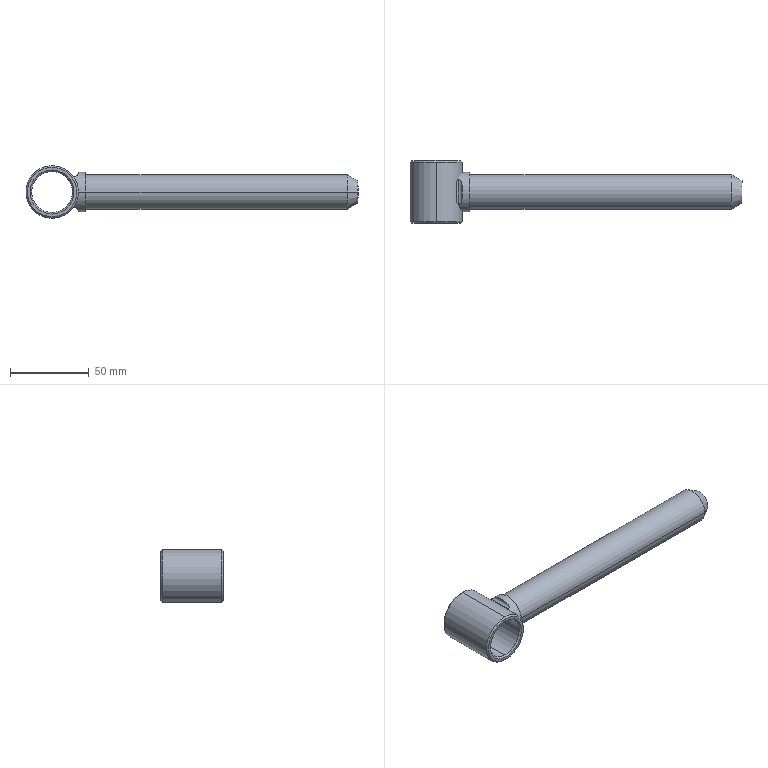Part | SolidWorks | features BaseBody 1 | 1 solid | 28 faces | box 211.2 x 40 x 33.4 mm | volume 81310 mm3 | cylinder 12 | cone 10 | plane 6 | commonest cylinder face diameters 4 x4 22 x2 25 x2 26.04 x2 33.4 x2
STEP:
#1=CARTESIAN_POINT('',(-54.286,20.854,0.));
#2=VERTEX_POINT('',#1);
#3=CARTESIAN_POINT('',(-54.286,-1.146,0.));
#4=VERTEX_POINT('',#3);
#5=CARTESIAN_POINT('',(-54.286,9.854,0.));
#6=DIRECTION('',(1.,0.,0.));
#7=DIRECTION('',(0.,1.,0.));
#8=AXIS2_PLACEMENT_3D('',#5,#6,#7);
#9=CIRCLE('',#8,11.);
#10=EDGE_CURVE('',#2,#4,#9,.T.);
#11=ORIENTED_EDGE('',*,*,#10,.T.);
#12=CARTESIAN_POINT('',(111.982,-1.146,0.));
#13=VERTEX_POINT('',#12);
#14=CARTESIAN_POINT('',(28.848,-1.146,0.));
#15=DIRECTION('',(1.,0.,0.));
#16=VECTOR('',#15,1000.);
#17=LINE('',#14,#16);
#18=EDGE_CURVE('',#4,#13,#17,.T.);
#19=ORIENTED_EDGE('',*,*,#18,.T.);
#20=CARTESIAN_POINT('',(111.982,20.854,0.));
#21=VERTEX_POINT('',#20);
#22=CARTESIAN_POINT('',(111.982,9.854,0.));
#23=DIRECTION('',(-1.,0.,0.));
#24=DIRECTION('',(0.,1.,0.));
#25=AXIS2_PLACEMENT_3D('',#22,#23,#24);
#26=CIRCLE('',#25,11.);
#27=EDGE_CURVE('',#13,#21,#26,.T.);
#28=ORIENTED_EDGE('',*,*,#27,.T.);
#29=CARTESIAN_POINT('',(28.848,20.854,0.));
#30=DIRECTION('',(1.,0.,0.));
#31=VECTOR('',#30,1000.);
#32=LINE('',#29,#31);
#33=EDGE_CURVE('',#2,#21,#32,.T.);
#34=ORIENTED_EDGE('',*,*,#33,.F.);
#35=EDGE_LOOP('',(#11,#19,#28,#34));
#36=FACE_OUTER_BOUND('',#35,.T.);
#37=CARTESIAN_POINT('',(28.848,9.854,0.));
#38=DIRECTION('',(1.,0.,0.));
#39=DIRECTION('',(0.,1.,0.));
#40=AXIS2_PLACEMENT_3D('',#37,#38,#39);
#41=CYLINDRICAL_SURFACE('',#40,11.);
#42=ADVANCED_FACE('',(#36),#41,.T.);
#43=CARTESIAN_POINT('',(118.714,2.741,0.));
#44=VERTEX_POINT('',#43);
#45=CARTESIAN_POINT('',(118.714,16.967,0.));
#46=VERTEX_POINT('',#45);
#47=CARTESIAN_POINT('',(118.714,9.854,0.));
#48=DIRECTION('',(-1.,0.,0.));
#49=DIRECTION('',(0.,-1.,0.));
#50=AXIS2_PLACEMENT_3D('',#47,#48,#49);
#51=CIRCLE('',#50,7.113);
#52=EDGE_CURVE('',#44,#46,#51,.T.);
#53=ORIENTED_EDGE('',*,*,#52,.T.);
#54=CARTESIAN_POINT('',(111.982,20.854,0.));
#55=DIRECTION('',(-0.866,0.5,0.));
#56=VECTOR('',#55,1000.);
#57=LINE('',#54,#56);
#58=EDGE_CURVE('',#46,#21,#57,.T.);
#59=ORIENTED_EDGE('',*,*,#58,.T.);
#60=ORIENTED_EDGE('',*,*,#27,.F.);
#61=CARTESIAN_POINT('',(111.982,-1.146,0.));
#62=DIRECTION('',(-0.866,-0.5,0.));
#63=VECTOR('',#62,1000.);
#64=LINE('',#61,#63);
#65=EDGE_CURVE('',#44,#13,#64,.T.);
#66=ORIENTED_EDGE('',*,*,#65,.F.);
#67=EDGE_LOOP('',(#53,#59,#60,#66));
#68=FACE_OUTER_BOUND('',#67,.T.);
#69=CARTESIAN_POINT('',(111.982,9.854,0.));
#70=DIRECTION('',(-1.,0.,0.));
#71=DIRECTION('',(0.,-1.,0.));
#72=AXIS2_PLACEMENT_3D('',#69,#70,#71);
#73=CONICAL_SURFACE('',#72,11.,0.5236);
#74=ADVANCED_FACE('',(#68),#73,.T.);
#75=CARTESIAN_POINT('',(-62.837,3.143,10.546));
#76=VERTEX_POINT('',#75);
#77=CARTESIAN_POINT('',(-59.086,-2.646,0.));
#78=VERTEX_POINT('',#77);
#79=CARTESIAN_POINT('',(-62.837,3.143,10.546));
#80=CARTESIAN_POINT('',(-62.392,2.286,10.));
#81=CARTESIAN_POINT('',(-61.935,1.517,9.368));
#82=CARTESIAN_POINT('',(-61.276,0.4757,8.279));
#83=CARTESIAN_POINT('',(-61.061,0.1469,7.892));
#84=CARTESIAN_POINT('',(-60.648,-0.4685,7.068));
#85=CARTESIAN_POINT('',(-60.454,-0.7505,6.638));
#86=CARTESIAN_POINT('',(-60.095,-1.263,5.738));
#87=CARTESIAN_POINT('',(-59.931,-1.494,5.269));
#88=CARTESIAN_POINT('',(-59.638,-1.9,4.288));
#89=CARTESIAN_POINT('',(-59.509,-2.075,3.774));
#90=CARTESIAN_POINT('',(-59.3,-2.358,2.722));
#91=CARTESIAN_POINT('',(-59.22,-2.466,2.181));
#92=CARTESIAN_POINT('',(-59.113,-2.61,1.096));
#93=CARTESIAN_POINT('',(-59.086,-2.646,0.5502));
#94=CARTESIAN_POINT('',(-59.086,-2.646,0.));
#95=B_SPLINE_CURVE_WITH_KNOTS('',3,(#79,#80,#81,#82,#83,#84,#85,#86,#87,#88,#89,#90,#91,#92,#93,#94),.UNSPECIFIED.,.F.,.F.,(4,2,2,2,2,2,2,4),(0.,0.003282,0.004923,0.006564,0.008205,0.009846,0.01149,0.01313),.UNSPECIFIED.);
#96=EDGE_CURVE('',#76,#78,#95,.T.);
#97=ORIENTED_EDGE('',*,*,#96,.T.);
#98=CARTESIAN_POINT('',(-54.286,-2.646,0.));
#99=VERTEX_POINT('',#98);
#100=CARTESIAN_POINT('',(-56.786,-2.646,0.));
#101=DIRECTION('',(1.,0.,0.));
#102=VECTOR('',#101,1000.);
#103=LINE('',#100,#102);
#104=EDGE_CURVE('',#78,#99,#103,.T.);
#105=ORIENTED_EDGE('',*,*,#104,.T.);
#106=CARTESIAN_POINT('',(-54.286,22.354,0.));
#107=VERTEX_POINT('',#106);
#108=CARTESIAN_POINT('',(-54.286,9.854,0.));
#109=DIRECTION('',(1.,0.,0.));
#110=DIRECTION('',(0.,1.,0.));
#111=AXIS2_PLACEMENT_3D('',#108,#109,#110);
#112=CIRCLE('',#111,12.5);
#113=EDGE_CURVE('',#107,#99,#112,.T.);
#114=ORIENTED_EDGE('',*,*,#113,.F.);
#115=CARTESIAN_POINT('',(-59.086,22.354,0.));
#116=VERTEX_POINT('',#115);
#117=CARTESIAN_POINT('',(-56.786,22.354,0.));
#118=DIRECTION('',(1.,0.,0.));
#119=VECTOR('',#118,1000.);
#120=LINE('',#117,#119);
#121=EDGE_CURVE('',#116,#107,#120,.T.);
#122=ORIENTED_EDGE('',*,*,#121,.F.);
#123=CARTESIAN_POINT('',(-62.837,16.565,10.546));
#124=VERTEX_POINT('',#123);
#125=CARTESIAN_POINT('',(-59.086,22.354,0.));
#126=CARTESIAN_POINT('',(-59.086,22.354,0.5493));
#127=CARTESIAN_POINT('',(-59.113,22.317,1.105));
#128=CARTESIAN_POINT('',(-59.222,22.172,2.197));
#129=CARTESIAN_POINT('',(-59.303,22.062,2.738));
#130=CARTESIAN_POINT('',(-59.614,21.64,4.301));
#131=CARTESIAN_POINT('',(-59.909,21.236,5.271));
#132=CARTESIAN_POINT('',(-60.452,20.461,6.634));
#133=CARTESIAN_POINT('',(-60.647,20.178,7.065));
#134=CARTESIAN_POINT('',(-61.055,19.57,7.881));
#135=CARTESIAN_POINT('',(-61.269,19.244,8.266));
#136=CARTESIAN_POINT('',(-61.709,18.549,8.995));
#137=CARTESIAN_POINT('',(-61.936,18.178,9.339));
#138=CARTESIAN_POINT('',(-62.389,17.4,9.978));
#139=CARTESIAN_POINT('',(-62.615,16.993,10.273));
#140=CARTESIAN_POINT('',(-62.837,16.565,10.546));
#141=B_SPLINE_CURVE_WITH_KNOTS('',3,(#125,#126,#127,#128,#129,#130,#131,#132,#133,#134,#135,#136,#137,#138,#139,#140),.UNSPECIFIED.,.F.,.F.,(4,2,2,2,2,2,2,4),(-0.00257,-0.0009334,0.0007035,0.003977,0.005614,0.007251,0.008888,0.01052),.UNSPECIFIED.);
#142=EDGE_CURVE('',#116,#124,#141,.T.);
#143=ORIENTED_EDGE('',*,*,#142,.T.);
#144=CARTESIAN_POINT('',(-61.286,17.603,9.808));
#145=VERTEX_POINT('',#144);
#146=CARTESIAN_POINT('',(-62.837,16.565,10.546));
#147=CARTESIAN_POINT('',(-62.765,16.703,10.458));
#148=CARTESIAN_POINT('',(-62.683,16.832,10.372));
#149=CARTESIAN_POINT('',(-62.49,17.072,10.206));
#150=CARTESIAN_POINT('',(-62.378,17.184,10.126));
#151=CARTESIAN_POINT('',(-62.115,17.379,9.982));
#152=CARTESIAN_POINT('',(-61.967,17.459,9.92));
#153=CARTESIAN_POINT('',(-61.722,17.544,9.855));
#154=CARTESIAN_POINT('',(-61.638,17.566,9.838));
#155=CARTESIAN_POINT('',(-61.465,17.595,9.815));
#156=CARTESIAN_POINT('',(-61.375,17.603,9.808));
#157=CARTESIAN_POINT('',(-61.286,17.603,9.808));
#158=B_SPLINE_CURVE_WITH_KNOTS('',3,(#146,#147,#148,#149,#150,#151,#152,#153,#154,#155,#156,#157),.UNSPECIFIED.,.F.,.F.,(4,2,2,2,2,4),(0.,0.0005249,0.00105,0.001575,0.001837,0.0021),.UNSPECIFIED.);
#159=EDGE_CURVE('',#124,#145,#158,.T.);
#160=ORIENTED_EDGE('',*,*,#159,.T.);
#161=CARTESIAN_POINT('',(-59.286,13.954,11.808));
#162=VERTEX_POINT('',#161);
#163=CARTESIAN_POINT('',(-61.286,17.603,9.808));
#164=CARTESIAN_POINT('',(-61.073,17.603,9.808));
#165=CARTESIAN_POINT('',(-60.861,17.558,9.844));
#166=CARTESIAN_POINT('',(-60.579,17.44,9.935));
#167=CARTESIAN_POINT('',(-60.489,17.392,9.972));
#168=CARTESIAN_POINT('',(-60.325,17.284,10.052));
#169=CARTESIAN_POINT('',(-60.249,17.225,10.096));
#170=CARTESIAN_POINT('',(-60.038,17.03,10.236));
#171=CARTESIAN_POINT('',(-59.922,16.882,10.339));
#172=CARTESIAN_POINT('',(-59.729,16.568,10.545));
#173=CARTESIAN_POINT('',(-59.65,16.399,10.651));
#174=CARTESIAN_POINT('',(-59.459,15.878,10.96));
#175=CARTESIAN_POINT('',(-59.387,15.512,11.154));
#176=CARTESIAN_POINT('',(-59.3,14.748,11.51));
#177=CARTESIAN_POINT('',(-59.286,14.355,11.669));
#178=CARTESIAN_POINT('',(-59.286,13.954,11.808));
#179=B_SPLINE_CURVE_WITH_KNOTS('',3,(#163,#164,#165,#166,#167,#168,#169,#170,#171,#172,#173,#174,#175,#176,#177,#178),.UNSPECIFIED.,.F.,.F.,(4,2,2,2,2,2,2,4),(0.0021,0.002728,0.003041,0.003355,0.003983,0.004611,0.005867,0.007122),.UNSPECIFIED.);
#180=EDGE_CURVE('',#145,#162,#179,.T.);
#181=ORIENTED_EDGE('',*,*,#180,.T.);
#182=CARTESIAN_POINT('',(-59.286,5.754,11.808));
#183=VERTEX_POINT('',#182);
#184=CARTESIAN_POINT('',(-59.286,9.854,0.));
#185=DIRECTION('',(1.,0.,0.));
#186=DIRECTION('',(0.,1.,0.));
#187=AXIS2_PLACEMENT_3D('',#184,#185,#186);
#188=CIRCLE('',#187,12.5);
#189=EDGE_CURVE('',#162,#183,#188,.T.);
#190=ORIENTED_EDGE('',*,*,#189,.T.);
#191=CARTESIAN_POINT('',(-61.286,2.105,9.808));
#192=VERTEX_POINT('',#191);
#193=CARTESIAN_POINT('',(-59.286,5.754,11.808));
#194=CARTESIAN_POINT('',(-59.286,5.354,11.669));
#195=CARTESIAN_POINT('',(-59.3,4.964,11.511));
#196=CARTESIAN_POINT('',(-59.385,4.209,11.161));
#197=CARTESIAN_POINT('',(-59.455,3.844,10.968));
#198=CARTESIAN_POINT('',(-59.646,3.317,10.657));
#199=CARTESIAN_POINT('',(-59.724,3.148,10.551));
#200=CARTESIAN_POINT('',(-59.916,2.834,10.344));
#201=CARTESIAN_POINT('',(-60.031,2.686,10.242));
#202=CARTESIAN_POINT('',(-60.243,2.488,10.1));
#203=CARTESIAN_POINT('',(-60.32,2.428,10.055));
#204=CARTESIAN_POINT('',(-60.485,2.318,9.973));
#205=CARTESIAN_POINT('',(-60.575,2.27,9.936));
#206=CARTESIAN_POINT('',(-60.764,2.19,9.875));
#207=CARTESIAN_POINT('',(-60.863,2.159,9.851));
#208=CARTESIAN_POINT('',(-61.072,2.116,9.817));
#209=CARTESIAN_POINT('',(-61.179,2.105,9.808));
#210=CARTESIAN_POINT('',(-61.286,2.105,9.808));
#211=B_SPLINE_CURVE_WITH_KNOTS('',3,(#193,#194,#195,#196,#197,#198,#199,#200,#201,#202,#203,#204,#205,#206,#207,#208,#209,#210),.UNSPECIFIED.,.F.,.F.,(4,2,2,2,2,2,2,2,4),(0.,0.001255,0.00251,0.003137,0.003765,0.004079,0.004392,0.004706,0.00502),.UNSPECIFIED.);
#212=EDGE_CURVE('',#183,#192,#211,.T.);
#213=ORIENTED_EDGE('',*,*,#212,.T.);
#214=CARTESIAN_POINT('',(-61.286,2.105,9.808));
#215=CARTESIAN_POINT('',(-61.462,2.105,9.808));
#216=CARTESIAN_POINT('',(-61.64,2.136,9.833));
#217=CARTESIAN_POINT('',(-61.965,2.248,9.92));
#218=CARTESIAN_POINT('',(-62.113,2.329,9.982));
#219=CARTESIAN_POINT('',(-62.374,2.521,10.124));
#220=CARTESIAN_POINT('',(-62.488,2.633,10.205));
#221=CARTESIAN_POINT('',(-62.682,2.875,10.371));
#222=CARTESIAN_POINT('',(-62.765,3.005,10.458));
#223=CARTESIAN_POINT('',(-62.837,3.143,10.546));
#224=B_SPLINE_CURVE_WITH_KNOTS('',3,(#214,#215,#216,#217,#218,#219,#220,#221,#222,#223),.UNSPECIFIED.,.F.,.F.,(4,2,2,2,4),(0.00502,0.005538,0.006055,0.006573,0.007091),.UNSPECIFIED.);
#225=EDGE_CURVE('',#192,#76,#224,.T.);
#226=ORIENTED_EDGE('',*,*,#225,.T.);
#227=EDGE_LOOP('',(#97,#105,#114,#122,#143,#160,#181,#190,#213,#226));
#228=FACE_OUTER_BOUND('',#227,.T.);
#229=CARTESIAN_POINT('',(-56.786,9.854,0.));
#230=DIRECTION('',(1.,0.,0.));
#231=DIRECTION('',(0.,1.,0.));
#232=AXIS2_PLACEMENT_3D('',#229,#230,#231);
#233=CYLINDRICAL_SURFACE('',#232,12.5);
#234=ADVANCED_FACE('',(#228),#233,.T.);
#235=CARTESIAN_POINT('',(-62.837,16.565,-10.546));
#236=VERTEX_POINT('',#235);
#237=CARTESIAN_POINT('',(-62.837,3.143,-10.546));
#238=VERTEX_POINT('',#237);
#239=CARTESIAN_POINT('',(-62.837,9.854,-10.546));
#240=DIRECTION('',(0.,-1.,0.));
#241=VECTOR('',#240,1000.);
#242=LINE('',#239,#241);
#243=EDGE_CURVE('',#236,#238,#242,.T.);
#244=ORIENTED_EDGE('',*,*,#243,.T.);
#245=CARTESIAN_POINT('',(-59.086,-2.646,0.));
#246=CARTESIAN_POINT('',(-59.086,-2.646,-0.5493));
#247=CARTESIAN_POINT('',(-59.113,-2.609,-1.105));
#248=CARTESIAN_POINT('',(-59.222,-2.464,-2.197));
#249=CARTESIAN_POINT('',(-59.303,-2.354,-2.738));
#250=CARTESIAN_POINT('',(-59.614,-1.932,-4.301));
#251=CARTESIAN_POINT('',(-59.909,-1.528,-5.271));
#252=CARTESIAN_POINT('',(-60.452,-0.753,-6.634));
#253=CARTESIAN_POINT('',(-60.647,-0.4702,-7.065));
#254=CARTESIAN_POINT('',(-61.055,0.138,-7.881));
#255=CARTESIAN_POINT('',(-61.269,0.4638,-8.266));
#256=CARTESIAN_POINT('',(-61.709,1.159,-8.995));
#257=CARTESIAN_POINT('',(-61.936,1.53,-9.339));
#258=CARTESIAN_POINT('',(-62.389,2.308,-9.978));
#259=CARTESIAN_POINT('',(-62.615,2.715,-10.273));
#260=CARTESIAN_POINT('',(-62.837,3.143,-10.546));
#261=B_SPLINE_CURVE_WITH_KNOTS('',3,(#245,#246,#247,#248,#249,#250,#251,#252,#253,#254,#255,#256,#257,#258,#259,#260),.UNSPECIFIED.,.F.,.F.,(4,2,2,2,2,2,2,4),(0.01313,0.01477,0.01641,0.01968,0.02132,0.02296,0.0246,0.02624),.UNSPECIFIED.);
#262=EDGE_CURVE('',#78,#238,#261,.T.);
#263=ORIENTED_EDGE('',*,*,#262,.F.);
#264=ORIENTED_EDGE('',*,*,#96,.F.);
#265=CARTESIAN_POINT('',(-62.837,9.854,10.546));
#266=DIRECTION('',(0.,1.,0.));
#267=VECTOR('',#266,1000.);
#268=LINE('',#265,#267);
#269=EDGE_CURVE('',#76,#124,#268,.T.);
#270=ORIENTED_EDGE('',*,*,#269,.T.);
#271=ORIENTED_EDGE('',*,*,#142,.F.);
#272=CARTESIAN_POINT('',(-62.837,16.565,-10.546));
#273=CARTESIAN_POINT('',(-62.392,17.422,-10.));
#274=CARTESIAN_POINT('',(-61.935,18.191,-9.368));
#275=CARTESIAN_POINT('',(-61.276,19.232,-8.279));
#276=CARTESIAN_POINT('',(-61.061,19.561,-7.892));
#277=CARTESIAN_POINT('',(-60.648,20.177,-7.068));
#278=CARTESIAN_POINT('',(-60.454,20.459,-6.638));
#279=CARTESIAN_POINT('',(-60.095,20.971,-5.738));
#280=CARTESIAN_POINT('',(-59.931,21.202,-5.269));
#281=CARTESIAN_POINT('',(-59.638,21.608,-4.288));
#282=CARTESIAN_POINT('',(-59.509,21.783,-3.774));
#283=CARTESIAN_POINT('',(-59.3,22.066,-2.722));
#284=CARTESIAN_POINT('',(-59.22,22.174,-2.181));
#285=CARTESIAN_POINT('',(-59.113,22.318,-1.096));
#286=CARTESIAN_POINT('',(-59.086,22.354,-0.5502));
#287=CARTESIAN_POINT('',(-59.086,22.354,0.));
#288=B_SPLINE_CURVE_WITH_KNOTS('',3,(#272,#273,#274,#275,#276,#277,#278,#279,#280,#281,#282,#283,#284,#285,#286,#287),.UNSPECIFIED.,.F.,.F.,(4,2,2,2,2,2,2,4),(-0.01569,-0.01241,-0.01077,-0.009129,-0.007489,-0.005849,-0.00421,-0.00257),.UNSPECIFIED.);
#289=EDGE_CURVE('',#236,#116,#288,.T.);
#290=ORIENTED_EDGE('',*,*,#289,.F.);
#291=EDGE_LOOP('',(#244,#263,#264,#270,#271,#290));
#292=FACE_BOUND('',#291,.T.);
#293=CARTESIAN_POINT('',(-75.786,-9.146,16.7));
#294=VERTEX_POINT('',#293);
#295=CARTESIAN_POINT('',(-75.786,-9.146,-16.7));
#296=VERTEX_POINT('',#295);
#297=CARTESIAN_POINT('',(-75.786,-9.146,0.));
#298=DIRECTION('',(0.,1.,0.));
#299=DIRECTION('',(0.,0.,1.));
#300=AXIS2_PLACEMENT_3D('',#297,#298,#299);
#301=CIRCLE('',#300,16.7);
#302=EDGE_CURVE('',#294,#296,#301,.T.);
#303=ORIENTED_EDGE('',*,*,#302,.T.);
#304=CARTESIAN_POINT('',(-75.786,28.854,-16.7));
#305=VERTEX_POINT('',#304);
#306=CARTESIAN_POINT('',(-75.786,9.854,-16.7));
#307=DIRECTION('',(0.,1.,0.));
#308=VECTOR('',#307,1000.);
#309=LINE('',#306,#308);
#310=EDGE_CURVE('',#296,#305,#309,.T.);
#311=ORIENTED_EDGE('',*,*,#310,.T.);
#312=CARTESIAN_POINT('',(-75.786,28.854,16.7));
#313=VERTEX_POINT('',#312);
#314=CARTESIAN_POINT('',(-75.786,28.854,0.));
#315=DIRECTION('',(0.,-1.,0.));
#316=DIRECTION('',(0.,0.,1.));
#317=AXIS2_PLACEMENT_3D('',#314,#315,#316);
#318=CIRCLE('',#317,16.7);
#319=EDGE_CURVE('',#305,#313,#318,.T.);
#320=ORIENTED_EDGE('',*,*,#319,.T.);
#321=CARTESIAN_POINT('',(-75.786,9.854,16.7));
#322=DIRECTION('',(0.,1.,0.));
#323=VECTOR('',#322,1000.);
#324=LINE('',#321,#323);
#325=EDGE_CURVE('',#294,#313,#324,.T.);
#326=ORIENTED_EDGE('',*,*,#325,.F.);
#327=EDGE_LOOP('',(#303,#311,#320,#326));
#328=FACE_OUTER_BOUND('',#327,.T.);
#329=CARTESIAN_POINT('',(-75.786,9.854,0.));
#330=DIRECTION('',(0.,1.,0.));
#331=DIRECTION('',(0.,0.,1.));
#332=AXIS2_PLACEMENT_3D('',#329,#330,#331);
#333=CYLINDRICAL_SURFACE('',#332,16.7);
#334=ADVANCED_FACE('',(#292,#328),#333,.T.);
#335=ORIENTED_EDGE('',*,*,#180,.F.);
#336=CARTESIAN_POINT('',(-61.286,9.854,9.808));
#337=DIRECTION('',(0.,-1.,0.));
#338=VECTOR('',#337,1000.);
#339=LINE('',#336,#338);
#340=EDGE_CURVE('',#145,#192,#339,.T.);
#341=ORIENTED_EDGE('',*,*,#340,.T.);
#342=ORIENTED_EDGE('',*,*,#212,.F.);
#343=CARTESIAN_POINT('',(-59.286,9.854,11.808));
#344=DIRECTION('',(0.,-1.,0.));
#345=VECTOR('',#344,1000.);
#346=LINE('',#343,#345);
#347=EDGE_CURVE('',#162,#183,#346,.T.);
#348=ORIENTED_EDGE('',*,*,#347,.F.);
#349=EDGE_LOOP('',(#335,#341,#342,#348));
#350=FACE_OUTER_BOUND('',#349,.T.);
#351=CARTESIAN_POINT('',(-61.286,9.854,11.808));
#352=DIRECTION('',(0.,-1.,0.));
#353=DIRECTION('',(0.,0.,-1.));
#354=AXIS2_PLACEMENT_3D('',#351,#352,#353);
#355=CYLINDRICAL_SURFACE('',#354,2.);
#356=ADVANCED_FACE('',(#350),#355,.F.);
#357=CARTESIAN_POINT('',(-61.286,2.105,-9.808));
#358=VERTEX_POINT('',#357);
#359=CARTESIAN_POINT('',(-59.286,5.754,-11.808));
#360=VERTEX_POINT('',#359);
#361=CARTESIAN_POINT('',(-61.286,2.105,-9.808));
#362=CARTESIAN_POINT('',(-61.073,2.105,-9.808));
#363=CARTESIAN_POINT('',(-60.861,2.15,-9.844));
#364=CARTESIAN_POINT('',(-60.579,2.268,-9.935));
#365=CARTESIAN_POINT('',(-60.489,2.316,-9.972));
#366=CARTESIAN_POINT('',(-60.325,2.424,-10.052));
#367=CARTESIAN_POINT('',(-60.249,2.483,-10.096));
#368=CARTESIAN_POINT('',(-60.038,2.678,-10.236));
#369=CARTESIAN_POINT('',(-59.922,2.826,-10.339));
#370=CARTESIAN_POINT('',(-59.729,3.14,-10.545));
#371=CARTESIAN_POINT('',(-59.65,3.309,-10.651));
#372=CARTESIAN_POINT('',(-59.459,3.83,-10.96));
#373=CARTESIAN_POINT('',(-59.387,4.196,-11.154));
#374=CARTESIAN_POINT('',(-59.3,4.96,-11.51));
#375=CARTESIAN_POINT('',(-59.286,5.353,-11.669));
#376=CARTESIAN_POINT('',(-59.286,5.754,-11.808));
#377=B_SPLINE_CURVE_WITH_KNOTS('',3,(#361,#362,#363,#364,#365,#366,#367,#368,#369,#370,#371,#372,#373,#374,#375,#376),.UNSPECIFIED.,.F.,.F.,(4,2,2,2,2,2,2,4),(0.0021,0.002728,0.003041,0.003355,0.003983,0.004611,0.005867,0.007122),.UNSPECIFIED.);
#378=EDGE_CURVE('',#358,#360,#377,.T.);
#379=ORIENTED_EDGE('',*,*,#378,.F.);
#380=CARTESIAN_POINT('',(-61.286,17.603,-9.808));
#381=VERTEX_POINT('',#380);
#382=CARTESIAN_POINT('',(-61.286,9.854,-9.808));
#383=DIRECTION('',(0.,1.,0.));
#384=VECTOR('',#383,1000.);
#385=LINE('',#382,#384);
#386=EDGE_CURVE('',#358,#381,#385,.T.);
#387=ORIENTED_EDGE('',*,*,#386,.T.);
#388=CARTESIAN_POINT('',(-59.286,13.954,-11.808));
#389=VERTEX_POINT('',#388);
#390=CARTESIAN_POINT('',(-59.286,13.954,-11.808));
#391=CARTESIAN_POINT('',(-59.286,14.354,-11.669));
#392=CARTESIAN_POINT('',(-59.3,14.744,-11.511));
#393=CARTESIAN_POINT('',(-59.385,15.499,-11.161));
#394=CARTESIAN_POINT('',(-59.455,15.864,-10.968));
#395=CARTESIAN_POINT('',(-59.646,16.391,-10.657));
#396=CARTESIAN_POINT('',(-59.724,16.56,-10.551));
#397=CARTESIAN_POINT('',(-59.916,16.874,-10.344));
#398=CARTESIAN_POINT('',(-60.031,17.022,-10.242));
#399=CARTESIAN_POINT('',(-60.243,17.22,-10.1));
#400=CARTESIAN_POINT('',(-60.32,17.28,-10.055));
#401=CARTESIAN_POINT('',(-60.485,17.39,-9.973));
#402=CARTESIAN_POINT('',(-60.575,17.438,-9.936));
#403=CARTESIAN_POINT('',(-60.764,17.518,-9.875));
#404=CARTESIAN_POINT('',(-60.863,17.549,-9.851));
#405=CARTESIAN_POINT('',(-61.072,17.592,-9.817));
#406=CARTESIAN_POINT('',(-61.179,17.603,-9.808));
#407=CARTESIAN_POINT('',(-61.286,17.603,-9.808));
#408=B_SPLINE_CURVE_WITH_KNOTS('',3,(#390,#391,#392,#393,#394,#395,#396,#397,#398,#399,#400,#401,#402,#403,#404,#405,#406,#407),.UNSPECIFIED.,.F.,.F.,(4,2,2,2,2,2,2,2,4),(0.,0.001255,0.00251,0.003137,0.003765,0.004079,0.004392,0.004706,0.00502),.UNSPECIFIED.);
#409=EDGE_CURVE('',#389,#381,#408,.T.);
#410=ORIENTED_EDGE('',*,*,#409,.F.);
#411=CARTESIAN_POINT('',(-59.286,9.854,-11.808));
#412=DIRECTION('',(0.,1.,0.));
#413=VECTOR('',#412,1000.);
#414=LINE('',#411,#413);
#415=EDGE_CURVE('',#360,#389,#414,.T.);
#416=ORIENTED_EDGE('',*,*,#415,.F.);
#417=EDGE_LOOP('',(#379,#387,#410,#416));
#418=FACE_OUTER_BOUND('',#417,.T.);
#419=CARTESIAN_POINT('',(-61.286,9.854,-11.808));
#420=DIRECTION('',(0.,1.,0.));
#421=DIRECTION('',(0.,0.,1.));
#422=AXIS2_PLACEMENT_3D('',#419,#420,#421);
#423=CYLINDRICAL_SURFACE('',#422,2.);
#424=ADVANCED_FACE('',(#418),#423,.F.);
#425=CARTESIAN_POINT('',(-75.786,-10.146,15.7));
#426=VERTEX_POINT('',#425);
#427=CARTESIAN_POINT('',(-75.786,-10.146,-15.7));
#428=VERTEX_POINT('',#427);
#429=CARTESIAN_POINT('',(-75.786,-10.146,0.));
#430=DIRECTION('',(0.,1.,0.));
#431=DIRECTION('',(0.,0.,1.));
#432=AXIS2_PLACEMENT_3D('',#429,#430,#431);
#433=CIRCLE('',#432,15.7);
#434=EDGE_CURVE('',#426,#428,#433,.T.);
#435=ORIENTED_EDGE('',*,*,#434,.T.);
#436=CARTESIAN_POINT('',(-75.786,-9.146,-16.7));
#437=DIRECTION('',(0.,0.7071,-0.7071));
#438=VECTOR('',#437,1000.);
#439=LINE('',#436,#438);
#440=EDGE_CURVE('',#428,#296,#439,.T.);
#441=ORIENTED_EDGE('',*,*,#440,.T.);
#442=ORIENTED_EDGE('',*,*,#302,.F.);
#443=CARTESIAN_POINT('',(-75.786,-9.146,16.7));
#444=DIRECTION('',(0.,0.7071,0.7071));
#445=VECTOR('',#444,1000.);
#446=LINE('',#443,#445);
#447=EDGE_CURVE('',#426,#294,#446,.T.);
#448=ORIENTED_EDGE('',*,*,#447,.F.);
#449=EDGE_LOOP('',(#435,#441,#442,#448));
#450=FACE_OUTER_BOUND('',#449,.T.);
#451=CARTESIAN_POINT('',(-75.786,-9.146,0.));
#452=DIRECTION('',(0.,1.,0.));
#453=DIRECTION('',(0.,0.,1.));
#454=AXIS2_PLACEMENT_3D('',#451,#452,#453);
#455=CONICAL_SURFACE('',#454,16.7,0.7854);
#456=ADVANCED_FACE('',(#450),#455,.T.);
#457=CARTESIAN_POINT('',(-75.786,29.854,-15.7));
#458=VERTEX_POINT('',#457);
#459=CARTESIAN_POINT('',(-75.786,29.854,15.7));
#460=VERTEX_POINT('',#459);
#461=CARTESIAN_POINT('',(-75.786,29.854,0.));
#462=DIRECTION('',(0.,-1.,0.));
#463=DIRECTION('',(0.,0.,-1.));
#464=AXIS2_PLACEMENT_3D('',#461,#462,#463);
#465=CIRCLE('',#464,15.7);
#466=EDGE_CURVE('',#458,#460,#465,.T.);
#467=ORIENTED_EDGE('',*,*,#466,.T.);
#468=CARTESIAN_POINT('',(-75.786,28.854,16.7));
#469=DIRECTION('',(0.,-0.7071,0.7071));
#470=VECTOR('',#469,1000.);
#471=LINE('',#468,#470);
#472=EDGE_CURVE('',#460,#313,#471,.T.);
#473=ORIENTED_EDGE('',*,*,#472,.T.);
#474=ORIENTED_EDGE('',*,*,#319,.F.);
#475=CARTESIAN_POINT('',(-75.786,28.854,-16.7));
#476=DIRECTION('',(0.,-0.7071,-0.7071));
#477=VECTOR('',#476,1000.);
#478=LINE('',#475,#477);
#479=EDGE_CURVE('',#458,#305,#478,.T.);
#480=ORIENTED_EDGE('',*,*,#479,.F.);
#481=EDGE_LOOP('',(#467,#473,#474,#480));
#482=FACE_OUTER_BOUND('',#481,.T.);
#483=CARTESIAN_POINT('',(-75.786,28.854,0.));
#484=DIRECTION('',(0.,-1.,0.));
#485=DIRECTION('',(0.,0.,-1.));
#486=AXIS2_PLACEMENT_3D('',#483,#484,#485);
#487=CONICAL_SURFACE('',#486,16.7,0.7854);
#488=ADVANCED_FACE('',(#482),#487,.T.);
#489=CARTESIAN_POINT('',(-75.786,-9.146,13.02));
#490=VERTEX_POINT('',#489);
#491=CARTESIAN_POINT('',(-75.786,-9.146,-13.02));
#492=VERTEX_POINT('',#491);
#493=CARTESIAN_POINT('',(-75.786,-9.146,0.));
#494=DIRECTION('',(0.,-1.,0.));
#495=DIRECTION('',(1.,0.,0.));
#496=AXIS2_PLACEMENT_3D('',#493,#494,#495);
#497=CIRCLE('',#496,13.02);
#498=EDGE_CURVE('',#490,#492,#497,.T.);
#499=ORIENTED_EDGE('',*,*,#498,.F.);
#500=CARTESIAN_POINT('',(-75.786,-10.146,14.02));
#501=VERTEX_POINT('',#500);
#502=CARTESIAN_POINT('',(-75.786,-10.146,14.02));
#503=DIRECTION('',(0.,-0.7071,0.7071));
#504=VECTOR('',#503,1000.);
#505=LINE('',#502,#504);
#506=EDGE_CURVE('',#490,#501,#505,.T.);
#507=ORIENTED_EDGE('',*,*,#506,.T.);
#508=CARTESIAN_POINT('',(-75.786,-10.146,-14.02));
#509=VERTEX_POINT('',#508);
#510=CARTESIAN_POINT('',(-75.786,-10.146,0.));
#511=DIRECTION('',(0.,1.,0.));
#512=DIRECTION('',(0.,0.,-1.));
#513=AXIS2_PLACEMENT_3D('',#510,#511,#512);
#514=CIRCLE('',#513,14.02);
#515=EDGE_CURVE('',#509,#501,#514,.T.);
#516=ORIENTED_EDGE('',*,*,#515,.F.);
#517=CARTESIAN_POINT('',(-75.786,-10.146,-14.02));
#518=DIRECTION('',(0.,-0.7071,-0.7071));
#519=VECTOR('',#518,1000.);
#520=LINE('',#517,#519);
#521=EDGE_CURVE('',#492,#509,#520,.T.);
#522=ORIENTED_EDGE('',*,*,#521,.F.);
#523=EDGE_LOOP('',(#499,#507,#516,#522));
#524=FACE_OUTER_BOUND('',#523,.T.);
#525=CARTESIAN_POINT('',(-75.786,-10.146,0.));
#526=DIRECTION('',(0.,-1.,0.));
#527=DIRECTION('',(0.,0.,-1.));
#528=AXIS2_PLACEMENT_3D('',#525,#526,#527);
#529=CONICAL_SURFACE('',#528,14.02,0.7854);
#530=ADVANCED_FACE('',(#524),#529,.F.);
#531=CARTESIAN_POINT('',(-75.786,28.854,-13.02));
#532=VERTEX_POINT('',#531);
#533=CARTESIAN_POINT('',(-75.786,28.854,13.02));
#534=VERTEX_POINT('',#533);
#535=CARTESIAN_POINT('',(-75.786,28.854,0.));
#536=DIRECTION('',(0.,1.,0.));
#537=DIRECTION('',(1.,0.,0.));
#538=AXIS2_PLACEMENT_3D('',#535,#536,#537);
#539=CIRCLE('',#538,13.02);
#540=EDGE_CURVE('',#532,#534,#539,.T.);
#541=ORIENTED_EDGE('',*,*,#540,.F.);
#542=CARTESIAN_POINT('',(-75.786,29.854,-14.02));
#543=VERTEX_POINT('',#542);
#544=CARTESIAN_POINT('',(-75.786,29.854,-14.02));
#545=DIRECTION('',(0.,0.7071,-0.7071));
#546=VECTOR('',#545,1000.);
#547=LINE('',#544,#546);
#548=EDGE_CURVE('',#532,#543,#547,.T.);
#549=ORIENTED_EDGE('',*,*,#548,.T.);
#550=CARTESIAN_POINT('',(-75.786,29.854,14.02));
#551=VERTEX_POINT('',#550);
#552=CARTESIAN_POINT('',(-75.786,29.854,0.));
#553=DIRECTION('',(0.,1.,0.));
#554=DIRECTION('',(0.,0.,1.));
#555=AXIS2_PLACEMENT_3D('',#552,#553,#554);
#556=CIRCLE('',#555,14.02);
#557=EDGE_CURVE('',#543,#551,#556,.T.);
#558=ORIENTED_EDGE('',*,*,#557,.T.);
#559=CARTESIAN_POINT('',(-75.786,29.854,14.02));
#560=DIRECTION('',(0.,0.7071,0.7071));
#561=VECTOR('',#560,1000.);
#562=LINE('',#559,#561);
#563=EDGE_CURVE('',#534,#551,#562,.T.);
#564=ORIENTED_EDGE('',*,*,#563,.F.);
#565=EDGE_LOOP('',(#541,#549,#558,#564));
#566=FACE_OUTER_BOUND('',#565,.T.);
#567=CARTESIAN_POINT('',(-75.786,29.854,0.));
#568=DIRECTION('',(0.,1.,0.));
#569=DIRECTION('',(0.,0.,1.));
#570=AXIS2_PLACEMENT_3D('',#567,#568,#569);
#571=CONICAL_SURFACE('',#570,14.02,0.7854);
#572=ADVANCED_FACE('',(#566),#571,.F.);
#573=ORIENTED_EDGE('',*,*,#498,.T.);
#574=CARTESIAN_POINT('',(-75.786,9.854,-13.02));
#575=DIRECTION('',(0.,1.,0.));
#576=VECTOR('',#575,1000.);
#577=LINE('',#574,#576);
#578=EDGE_CURVE('',#492,#532,#577,.T.);
#579=ORIENTED_EDGE('',*,*,#578,.T.);
#580=ORIENTED_EDGE('',*,*,#540,.T.);
#581=CARTESIAN_POINT('',(-75.786,9.854,13.02));
#582=DIRECTION('',(0.,1.,0.));
#583=VECTOR('',#582,1000.);
#584=LINE('',#581,#583);
#585=EDGE_CURVE('',#490,#534,#584,.T.);
#586=ORIENTED_EDGE('',*,*,#585,.F.);
#587=EDGE_LOOP('',(#573,#579,#580,#586));
#588=FACE_OUTER_BOUND('',#587,.T.);
#589=CARTESIAN_POINT('',(-75.786,9.854,0.));
#590=DIRECTION('',(0.,1.,0.));
#591=DIRECTION('',(0.,0.,1.));
#592=AXIS2_PLACEMENT_3D('',#589,#590,#591);
#593=CYLINDRICAL_SURFACE('',#592,13.02);
#594=ADVANCED_FACE('',(#588),#593,.F.);
#595=ORIENTED_EDGE('',*,*,#18,.F.);
#596=CARTESIAN_POINT('',(-54.286,9.854,0.));
#597=DIRECTION('',(1.,0.,0.));
#598=DIRECTION('',(0.,1.,0.));
#599=AXIS2_PLACEMENT_3D('',#596,#597,#598);
#600=CIRCLE('',#599,11.);
#601=EDGE_CURVE('',#4,#2,#600,.T.);
#602=ORIENTED_EDGE('',*,*,#601,.T.);
#603=ORIENTED_EDGE('',*,*,#33,.T.);
#604=CARTESIAN_POINT('',(111.982,9.854,0.));
#605=DIRECTION('',(-1.,0.,0.));
#606=DIRECTION('',(0.,1.,0.));
#607=AXIS2_PLACEMENT_3D('',#604,#605,#606);
#608=CIRCLE('',#607,11.);
#609=EDGE_CURVE('',#21,#13,#608,.T.);
#610=ORIENTED_EDGE('',*,*,#609,.T.);
#611=EDGE_LOOP('',(#595,#602,#603,#610));
#612=FACE_OUTER_BOUND('',#611,.T.);
#613=CARTESIAN_POINT('',(28.848,9.854,0.));
#614=DIRECTION('',(1.,0.,0.));
#615=DIRECTION('',(0.,1.,0.));
#616=AXIS2_PLACEMENT_3D('',#613,#614,#615);
#617=CYLINDRICAL_SURFACE('',#616,11.);
#618=ADVANCED_FACE('',(#612),#617,.T.);
#619=ORIENTED_EDGE('',*,*,#10,.F.);
#620=ORIENTED_EDGE('',*,*,#601,.F.);
#621=EDGE_LOOP('',(#619,#620));
#622=FACE_BOUND('',#621,.T.);
#623=ORIENTED_EDGE('',*,*,#113,.T.);
#624=CARTESIAN_POINT('',(-54.286,9.854,0.));
#625=DIRECTION('',(1.,0.,0.));
#626=DIRECTION('',(0.,1.,0.));
#627=AXIS2_PLACEMENT_3D('',#624,#625,#626);
#628=CIRCLE('',#627,12.5);
#629=EDGE_CURVE('',#99,#107,#628,.T.);
#630=ORIENTED_EDGE('',*,*,#629,.T.);
#631=EDGE_LOOP('',(#623,#630));
#632=FACE_OUTER_BOUND('',#631,.T.);
#633=CARTESIAN_POINT('',(-54.286,21.604,0.));
#634=DIRECTION('',(1.,0.,0.));
#635=DIRECTION('',(0.,1.,0.));
#636=AXIS2_PLACEMENT_3D('',#633,#634,#635);
#637=PLANE('',#636);
#638=ADVANCED_FACE('',(#622,#632),#637,.T.);
#639=ORIENTED_EDGE('',*,*,#58,.F.);
#640=CARTESIAN_POINT('',(118.714,9.854,0.));
#641=DIRECTION('',(-1.,0.,0.));
#642=DIRECTION('',(0.,-1.,0.));
#643=AXIS2_PLACEMENT_3D('',#640,#641,#642);
#644=CIRCLE('',#643,7.113);
#645=EDGE_CURVE('',#46,#44,#644,.T.);
#646=ORIENTED_EDGE('',*,*,#645,.T.);
#647=ORIENTED_EDGE('',*,*,#65,.T.);
#648=ORIENTED_EDGE('',*,*,#609,.F.);
#649=EDGE_LOOP('',(#639,#646,#647,#648));
#650=FACE_OUTER_BOUND('',#649,.T.);
#651=CARTESIAN_POINT('',(111.982,9.854,0.));
#652=DIRECTION('',(-1.,0.,0.));
#653=DIRECTION('',(0.,-1.,0.));
#654=AXIS2_PLACEMENT_3D('',#651,#652,#653);
#655=CONICAL_SURFACE('',#654,11.,0.5236);
#656=ADVANCED_FACE('',(#650),#655,.T.);
#657=ORIENTED_EDGE('',*,*,#104,.F.);
#658=ORIENTED_EDGE('',*,*,#262,.T.);
#659=CARTESIAN_POINT('',(-62.837,3.143,-10.546));
#660=CARTESIAN_POINT('',(-62.765,3.005,-10.458));
#661=CARTESIAN_POINT('',(-62.683,2.876,-10.372));
#662=CARTESIAN_POINT('',(-62.49,2.636,-10.206));
#663=CARTESIAN_POINT('',(-62.378,2.524,-10.126));
#664=CARTESIAN_POINT('',(-62.115,2.329,-9.982));
#665=CARTESIAN_POINT('',(-61.967,2.249,-9.92));
#666=CARTESIAN_POINT('',(-61.722,2.164,-9.855));
#667=CARTESIAN_POINT('',(-61.638,2.142,-9.838));
#668=CARTESIAN_POINT('',(-61.465,2.113,-9.815));
#669=CARTESIAN_POINT('',(-61.375,2.105,-9.808));
#670=CARTESIAN_POINT('',(-61.286,2.105,-9.808));
#671=B_SPLINE_CURVE_WITH_KNOTS('',3,(#659,#660,#661,#662,#663,#664,#665,#666,#667,#668,#669,#670),.UNSPECIFIED.,.F.,.F.,(4,2,2,2,2,4),(0.,0.0005249,0.00105,0.001575,0.001837,0.0021),.UNSPECIFIED.);
#672=EDGE_CURVE('',#238,#358,#671,.T.);
#673=ORIENTED_EDGE('',*,*,#672,.T.);
#674=ORIENTED_EDGE('',*,*,#378,.T.);
#675=CARTESIAN_POINT('',(-59.286,9.854,0.));
#676=DIRECTION('',(1.,0.,0.));
#677=DIRECTION('',(0.,1.,0.));
#678=AXIS2_PLACEMENT_3D('',#675,#676,#677);
#679=CIRCLE('',#678,12.5);
#680=EDGE_CURVE('',#360,#389,#679,.T.);
#681=ORIENTED_EDGE('',*,*,#680,.T.);
#682=ORIENTED_EDGE('',*,*,#409,.T.);
#683=CARTESIAN_POINT('',(-61.286,17.603,-9.808));
#684=CARTESIAN_POINT('',(-61.462,17.603,-9.808));
#685=CARTESIAN_POINT('',(-61.64,17.572,-9.833));
#686=CARTESIAN_POINT('',(-61.965,17.46,-9.92));
#687=CARTESIAN_POINT('',(-62.113,17.379,-9.982));
#688=CARTESIAN_POINT('',(-62.374,17.187,-10.124));
#689=CARTESIAN_POINT('',(-62.488,17.075,-10.205));
#690=CARTESIAN_POINT('',(-62.682,16.833,-10.371));
#691=CARTESIAN_POINT('',(-62.765,16.703,-10.458));
#692=CARTESIAN_POINT('',(-62.837,16.565,-10.546));
#693=B_SPLINE_CURVE_WITH_KNOTS('',3,(#683,#684,#685,#686,#687,#688,#689,#690,#691,#692),.UNSPECIFIED.,.F.,.F.,(4,2,2,2,4),(0.00502,0.005538,0.006055,0.006573,0.007091),.UNSPECIFIED.);
#694=EDGE_CURVE('',#381,#236,#693,.T.);
#695=ORIENTED_EDGE('',*,*,#694,.T.);
#696=ORIENTED_EDGE('',*,*,#289,.T.);
#697=ORIENTED_EDGE('',*,*,#121,.T.);
#698=ORIENTED_EDGE('',*,*,#629,.F.);
#699=EDGE_LOOP('',(#657,#658,#673,#674,#681,#682,#695,#696,#697,#698));
#700=FACE_OUTER_BOUND('',#699,.T.);
#701=CARTESIAN_POINT('',(-56.786,9.854,0.));
#702=DIRECTION('',(1.,0.,0.));
#703=DIRECTION('',(0.,1.,0.));
#704=AXIS2_PLACEMENT_3D('',#701,#702,#703);
#705=CYLINDRICAL_SURFACE('',#704,12.5);
#706=ADVANCED_FACE('',(#700),#705,.T.);
#707=ORIENTED_EDGE('',*,*,#52,.F.);
#708=ORIENTED_EDGE('',*,*,#645,.F.);
#709=EDGE_LOOP('',(#707,#708));
#710=FACE_OUTER_BOUND('',#709,.T.);
#711=CARTESIAN_POINT('',(118.714,13.411,0.));
#712=DIRECTION('',(1.,0.,0.));
#713=DIRECTION('',(0.,1.,0.));
#714=AXIS2_PLACEMENT_3D('',#711,#712,#713);
#715=PLANE('',#714);
#716=ADVANCED_FACE('',(#710),#715,.T.);
#717=ORIENTED_EDGE('',*,*,#310,.F.);
#718=CARTESIAN_POINT('',(-75.786,-9.146,0.));
#719=DIRECTION('',(0.,1.,0.));
#720=DIRECTION('',(0.,0.,1.));
#721=AXIS2_PLACEMENT_3D('',#718,#719,#720);
#722=CIRCLE('',#721,16.7);
#723=EDGE_CURVE('',#296,#294,#722,.T.);
#724=ORIENTED_EDGE('',*,*,#723,.T.);
#725=ORIENTED_EDGE('',*,*,#325,.T.);
#726=CARTESIAN_POINT('',(-75.786,28.854,0.));
#727=DIRECTION('',(0.,-1.,0.));
#728=DIRECTION('',(0.,0.,1.));
#729=AXIS2_PLACEMENT_3D('',#726,#727,#728);
#730=CIRCLE('',#729,16.7);
#731=EDGE_CURVE('',#313,#305,#730,.T.);
#732=ORIENTED_EDGE('',*,*,#731,.T.);
#733=EDGE_LOOP('',(#717,#724,#725,#732));
#734=FACE_OUTER_BOUND('',#733,.T.);
#735=CARTESIAN_POINT('',(-75.786,9.854,0.));
#736=DIRECTION('',(0.,1.,0.));
#737=DIRECTION('',(0.,0.,1.));
#738=AXIS2_PLACEMENT_3D('',#735,#736,#737);
#739=CYLINDRICAL_SURFACE('',#738,16.7);
#740=ADVANCED_FACE('',(#734),#739,.T.);
#741=ORIENTED_EDGE('',*,*,#340,.F.);
#742=ORIENTED_EDGE('',*,*,#159,.F.);
#743=ORIENTED_EDGE('',*,*,#269,.F.);
#744=ORIENTED_EDGE('',*,*,#225,.F.);
#745=EDGE_LOOP('',(#741,#742,#743,#744));
#746=FACE_OUTER_BOUND('',#745,.T.);
#747=CARTESIAN_POINT('',(-61.286,9.854,11.808));
#748=DIRECTION('',(0.,-1.,0.));
#749=DIRECTION('',(0.,0.,-1.));
#750=AXIS2_PLACEMENT_3D('',#747,#748,#749);
#751=CYLINDRICAL_SURFACE('',#750,2.);
#752=ADVANCED_FACE('',(#746),#751,.F.);
#753=ORIENTED_EDGE('',*,*,#347,.T.);
#754=ORIENTED_EDGE('',*,*,#189,.F.);
#755=EDGE_LOOP('',(#753,#754));
#756=FACE_OUTER_BOUND('',#755,.T.);
#757=CARTESIAN_POINT('',(-59.286,16.104,0.));
#758=DIRECTION('',(-1.,0.,0.));
#759=DIRECTION('',(0.,-1.,0.));
#760=AXIS2_PLACEMENT_3D('',#757,#758,#759);
#761=PLANE('',#760);
#762=ADVANCED_FACE('',(#756),#761,.T.);
#763=ORIENTED_EDGE('',*,*,#386,.F.);
#764=ORIENTED_EDGE('',*,*,#672,.F.);
#765=ORIENTED_EDGE('',*,*,#243,.F.);
#766=ORIENTED_EDGE('',*,*,#694,.F.);
#767=EDGE_LOOP('',(#763,#764,#765,#766));
#768=FACE_OUTER_BOUND('',#767,.T.);
#769=CARTESIAN_POINT('',(-61.286,9.854,-11.808));
#770=DIRECTION('',(0.,1.,0.));
#771=DIRECTION('',(0.,0.,1.));
#772=AXIS2_PLACEMENT_3D('',#769,#770,#771);
#773=CYLINDRICAL_SURFACE('',#772,2.);
#774=ADVANCED_FACE('',(#768),#773,.F.);
#775=ORIENTED_EDGE('',*,*,#415,.T.);
#776=ORIENTED_EDGE('',*,*,#680,.F.);
#777=EDGE_LOOP('',(#775,#776));
#778=FACE_OUTER_BOUND('',#777,.T.);
#779=CARTESIAN_POINT('',(-59.286,16.104,0.));
#780=DIRECTION('',(-1.,0.,0.));
#781=DIRECTION('',(0.,-1.,0.));
#782=AXIS2_PLACEMENT_3D('',#779,#780,#781);
#783=PLANE('',#782);
#784=ADVANCED_FACE('',(#778),#783,.T.);
#785=ORIENTED_EDGE('',*,*,#440,.F.);
#786=CARTESIAN_POINT('',(-75.786,-10.146,0.));
#787=DIRECTION('',(0.,1.,0.));
#788=DIRECTION('',(0.,0.,1.));
#789=AXIS2_PLACEMENT_3D('',#786,#787,#788);
#790=CIRCLE('',#789,15.7);
#791=EDGE_CURVE('',#428,#426,#790,.T.);
#792=ORIENTED_EDGE('',*,*,#791,.T.);
#793=ORIENTED_EDGE('',*,*,#447,.T.);
#794=ORIENTED_EDGE('',*,*,#723,.F.);
#795=EDGE_LOOP('',(#785,#792,#793,#794));
#796=FACE_OUTER_BOUND('',#795,.T.);
#797=CARTESIAN_POINT('',(-75.786,-9.146,0.));
#798=DIRECTION('',(0.,1.,0.));
#799=DIRECTION('',(0.,0.,1.));
#800=AXIS2_PLACEMENT_3D('',#797,#798,#799);
#801=CONICAL_SURFACE('',#800,16.7,0.7854);
#802=ADVANCED_FACE('',(#796),#801,.T.);
#803=ORIENTED_EDGE('',*,*,#472,.F.);
#804=CARTESIAN_POINT('',(-75.786,29.854,0.));
#805=DIRECTION('',(0.,-1.,0.));
#806=DIRECTION('',(0.,0.,-1.));
#807=AXIS2_PLACEMENT_3D('',#804,#805,#806);
#808=CIRCLE('',#807,15.7);
#809=EDGE_CURVE('',#460,#458,#808,.T.);
#810=ORIENTED_EDGE('',*,*,#809,.T.);
#811=ORIENTED_EDGE('',*,*,#479,.T.);
#812=ORIENTED_EDGE('',*,*,#731,.F.);
#813=EDGE_LOOP('',(#803,#810,#811,#812));
#814=FACE_OUTER_BOUND('',#813,.T.);
#815=CARTESIAN_POINT('',(-75.786,28.854,0.));
#816=DIRECTION('',(0.,-1.,0.));
#817=DIRECTION('',(0.,0.,-1.));
#818=AXIS2_PLACEMENT_3D('',#815,#816,#817);
#819=CONICAL_SURFACE('',#818,16.7,0.7854);
#820=ADVANCED_FACE('',(#814),#819,.T.);
#821=ORIENTED_EDGE('',*,*,#515,.T.);
#822=CARTESIAN_POINT('',(-75.786,-10.146,0.));
#823=DIRECTION('',(0.,1.,0.));
#824=DIRECTION('',(0.,0.,-1.));
#825=AXIS2_PLACEMENT_3D('',#822,#823,#824);
#826=CIRCLE('',#825,14.02);
#827=EDGE_CURVE('',#501,#509,#826,.T.);
#828=ORIENTED_EDGE('',*,*,#827,.T.);
#829=EDGE_LOOP('',(#821,#828));
#830=FACE_BOUND('',#829,.T.);
#831=ORIENTED_EDGE('',*,*,#434,.F.);
#832=ORIENTED_EDGE('',*,*,#791,.F.);
#833=EDGE_LOOP('',(#831,#832));
#834=FACE_OUTER_BOUND('',#833,.T.);
#835=CARTESIAN_POINT('',(-75.786,-10.146,0.));
#836=DIRECTION('',(0.,-1.,0.));
#837=DIRECTION('',(0.,0.,-1.));
#838=AXIS2_PLACEMENT_3D('',#835,#836,#837);
#839=PLANE('',#838);
#840=ADVANCED_FACE('',(#830,#834),#839,.T.);
#841=CARTESIAN_POINT('',(-75.786,29.854,0.));
#842=DIRECTION('',(0.,1.,0.));
#843=DIRECTION('',(0.,0.,1.));
#844=AXIS2_PLACEMENT_3D('',#841,#842,#843);
#845=CIRCLE('',#844,14.02);
#846=EDGE_CURVE('',#551,#543,#845,.T.);
#847=ORIENTED_EDGE('',*,*,#846,.F.);
#848=ORIENTED_EDGE('',*,*,#557,.F.);
#849=EDGE_LOOP('',(#847,#848));
#850=FACE_BOUND('',#849,.T.);
#851=ORIENTED_EDGE('',*,*,#466,.F.);
#852=ORIENTED_EDGE('',*,*,#809,.F.);
#853=EDGE_LOOP('',(#851,#852));
#854=FACE_OUTER_BOUND('',#853,.T.);
#855=CARTESIAN_POINT('',(-75.786,29.854,0.));
#856=DIRECTION('',(0.,-1.,0.));
#857=DIRECTION('',(0.,0.,-1.));
#858=AXIS2_PLACEMENT_3D('',#855,#856,#857);
#859=PLANE('',#858);
#860=ADVANCED_FACE('',(#850,#854),#859,.F.);
#861=ORIENTED_EDGE('',*,*,#506,.F.);
#862=CARTESIAN_POINT('',(-75.786,-9.146,0.));
#863=DIRECTION('',(0.,-1.,0.));
#864=DIRECTION('',(1.,0.,0.));
#865=AXIS2_PLACEMENT_3D('',#862,#863,#864);
#866=CIRCLE('',#865,13.02);
#867=EDGE_CURVE('',#492,#490,#866,.T.);
#868=ORIENTED_EDGE('',*,*,#867,.F.);
#869=ORIENTED_EDGE('',*,*,#521,.T.);
#870=ORIENTED_EDGE('',*,*,#827,.F.);
#871=EDGE_LOOP('',(#861,#868,#869,#870));
#872=FACE_OUTER_BOUND('',#871,.T.);
#873=CARTESIAN_POINT('',(-75.786,-10.146,0.));
#874=DIRECTION('',(0.,-1.,0.));
#875=DIRECTION('',(0.,0.,-1.));
#876=AXIS2_PLACEMENT_3D('',#873,#874,#875);
#877=CONICAL_SURFACE('',#876,14.02,0.7854);
#878=ADVANCED_FACE('',(#872),#877,.F.);
#879=ORIENTED_EDGE('',*,*,#548,.F.);
#880=CARTESIAN_POINT('',(-75.786,28.854,0.));
#881=DIRECTION('',(0.,1.,0.));
#882=DIRECTION('',(1.,0.,0.));
#883=AXIS2_PLACEMENT_3D('',#880,#881,#882);
#884=CIRCLE('',#883,13.02);
#885=EDGE_CURVE('',#534,#532,#884,.T.);
#886=ORIENTED_EDGE('',*,*,#885,.F.);
#887=ORIENTED_EDGE('',*,*,#563,.T.);
#888=ORIENTED_EDGE('',*,*,#846,.T.);
#889=EDGE_LOOP('',(#879,#886,#887,#888));
#890=FACE_OUTER_BOUND('',#889,.T.);
#891=CARTESIAN_POINT('',(-75.786,29.854,0.));
#892=DIRECTION('',(0.,1.,0.));
#893=DIRECTION('',(0.,0.,1.));
#894=AXIS2_PLACEMENT_3D('',#891,#892,#893);
#895=CONICAL_SURFACE('',#894,14.02,0.7854);
#896=ADVANCED_FACE('',(#890),#895,.F.);
#897=ORIENTED_EDGE('',*,*,#578,.F.);
#898=ORIENTED_EDGE('',*,*,#867,.T.);
#899=ORIENTED_EDGE('',*,*,#585,.T.);
#900=ORIENTED_EDGE('',*,*,#885,.T.);
#901=EDGE_LOOP('',(#897,#898,#899,#900));
#902=FACE_OUTER_BOUND('',#901,.T.);
#903=CARTESIAN_POINT('',(-75.786,9.854,0.));
#904=DIRECTION('',(0.,1.,0.));
#905=DIRECTION('',(0.,0.,1.));
#906=AXIS2_PLACEMENT_3D('',#903,#904,#905);
#907=CYLINDRICAL_SURFACE('',#906,13.02);
#908=ADVANCED_FACE('',(#902),#907,.F.);
#909=CLOSED_SHELL('',(#42,#74,#234,#334,#356,#424,#456,#488,#530,#572,#594,#618,#638,#656,#706,#716,#740,#752,#762,#774,#784,#802,#820,#840,#860,#878,#896,#908));
#910=MANIFOLD_SOLID_BREP('',#909);
#911=CARTESIAN_POINT('',(0.,0.,0.));
#912=DIRECTION('',(0.,0.,1.));
#913=DIRECTION('',(1.,0.,0.));
#914=AXIS2_PLACEMENT_3D('',#911,#912,#913);
#915=(LENGTH_UNIT()NAMED_UNIT(*)SI_UNIT(.MILLI.,.METRE.));
#916=UNCERTAINTY_MEASURE_WITH_UNIT(LENGTH_MEASURE(0.00001),#915,'','');
#917=(NAMED_UNIT(*)PLANE_ANGLE_UNIT()SI_UNIT($,.RADIAN.));
#918=(NAMED_UNIT(*)SI_UNIT($,.STERADIAN.)SOLID_ANGLE_UNIT());
#919=(GEOMETRIC_REPRESENTATION_CONTEXT(3)GLOBAL_UNCERTAINTY_ASSIGNED_CONTEXT((#916))GLOBAL_UNIT_ASSIGNED_CONTEXT((#915,#917,#918))REPRESENTATION_CONTEXT('',''));
#920=ADVANCED_BREP_SHAPE_REPRESENTATION('',(#910,#914),#919);